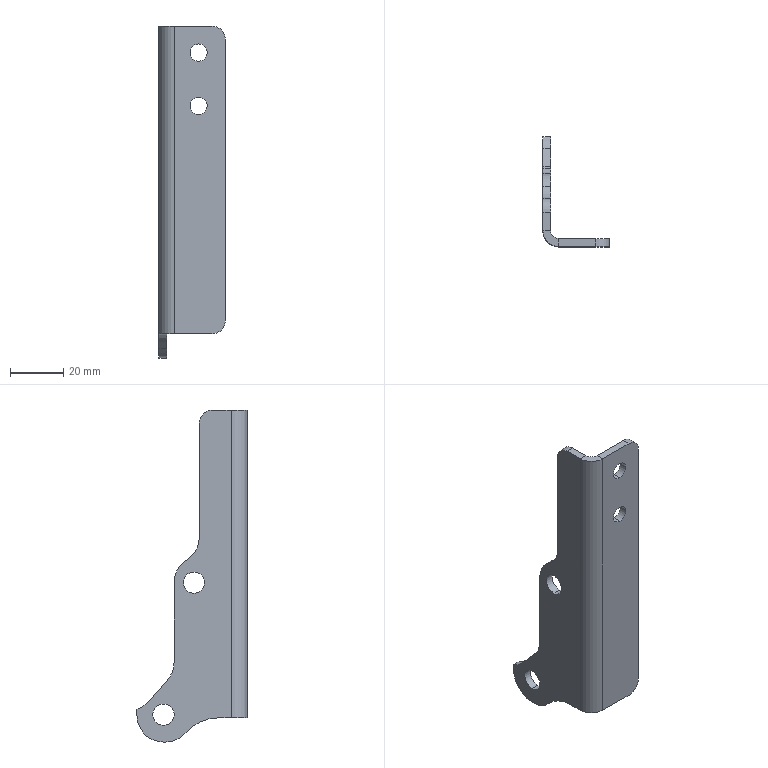Part | SolidWorks | features BaseBody 1 | 1 solid | 37 faces | box 25 x 41.473 x 125 mm | volume 15257 mm3 | cylinder 21 | plane 16 | commonest cylinder face diameters 20 x6 6.5 x4 8 x4 10 x3 6 x1 12 x1
STEP:
#1=CARTESIAN_POINT('',(0.,30.37,-102.09));
#2=VERTEX_POINT('',#1);
#3=CARTESIAN_POINT('',(3.,30.37,-102.09));
#4=VERTEX_POINT('',#3);
#5=CARTESIAN_POINT('',(3.,30.37,-102.09));
#6=DIRECTION('',(1.,0.,0.));
#7=VECTOR('',#6,1000.);
#8=LINE('',#5,#7);
#9=EDGE_CURVE('',#2,#4,#8,.T.);
#10=ORIENTED_EDGE('',*,*,#9,.T.);
#11=CARTESIAN_POINT('',(3.,37.101,-109.825));
#12=VERTEX_POINT('',#11);
#13=CARTESIAN_POINT('',(3.,28.627,-100.088));
#14=DIRECTION('',(0.,0.6565,-0.7544));
#15=VECTOR('',#14,1000.);
#16=LINE('',#13,#15);
#17=EDGE_CURVE('',#4,#12,#16,.T.);
#18=ORIENTED_EDGE('',*,*,#17,.T.);
#19=CARTESIAN_POINT('',(0.,37.101,-109.825));
#20=VERTEX_POINT('',#19);
#21=CARTESIAN_POINT('',(10.,37.101,-109.825));
#22=DIRECTION('',(-1.,0.,0.));
#23=VECTOR('',#22,1000.);
#24=LINE('',#21,#23);
#25=EDGE_CURVE('',#12,#20,#24,.T.);
#26=ORIENTED_EDGE('',*,*,#25,.T.);
#27=CARTESIAN_POINT('',(0.,29.519,-101.113));
#28=DIRECTION('',(0.,0.6565,-0.7544));
#29=VECTOR('',#28,1000.);
#30=LINE('',#27,#29);
#31=EDGE_CURVE('',#2,#20,#30,.T.);
#32=ORIENTED_EDGE('',*,*,#31,.F.);
#33=EDGE_LOOP('',(#10,#18,#26,#32));
#34=FACE_OUTER_BOUND('',#33,.T.);
#35=CARTESIAN_POINT('',(10.,29.519,-101.113));
#36=DIRECTION('',(0.,-0.7544,-0.6565));
#37=DIRECTION('',(0.,0.6565,-0.7544));
#38=AXIS2_PLACEMENT_3D('',#35,#36,#37);
#39=PLANE('',#38);
#40=ADVANCED_FACE('',(#34),#39,.F.);
#41=CARTESIAN_POINT('',(0.,18.,-5.));
#42=VERTEX_POINT('',#41);
#43=CARTESIAN_POINT('',(0.,13.,0.));
#44=VERTEX_POINT('',#43);
#45=CARTESIAN_POINT('',(0.,13.,-5.));
#46=DIRECTION('',(1.,0.,0.));
#47=DIRECTION('',(0.,0.,-1.));
#48=AXIS2_PLACEMENT_3D('',#45,#46,#47);
#49=CIRCLE('',#48,5.);
#50=EDGE_CURVE('',#42,#44,#49,.T.);
#51=ORIENTED_EDGE('',*,*,#50,.T.);
#52=CARTESIAN_POINT('',(3.,13.,0.));
#53=VERTEX_POINT('',#52);
#54=CARTESIAN_POINT('',(6.,13.,0.));
#55=DIRECTION('',(1.,0.,0.));
#56=VECTOR('',#55,1000.);
#57=LINE('',#54,#56);
#58=EDGE_CURVE('',#44,#53,#57,.T.);
#59=ORIENTED_EDGE('',*,*,#58,.T.);
#60=CARTESIAN_POINT('',(3.,18.,-5.));
#61=VERTEX_POINT('',#60);
#62=CARTESIAN_POINT('',(3.,13.,-5.));
#63=DIRECTION('',(-1.,0.,0.));
#64=DIRECTION('',(0.,0.,-1.));
#65=AXIS2_PLACEMENT_3D('',#62,#63,#64);
#66=CIRCLE('',#65,5.);
#67=EDGE_CURVE('',#53,#61,#66,.T.);
#68=ORIENTED_EDGE('',*,*,#67,.T.);
#69=CARTESIAN_POINT('',(-7.,18.,-5.));
#70=DIRECTION('',(-1.,0.,0.));
#71=VECTOR('',#70,1000.);
#72=LINE('',#69,#71);
#73=EDGE_CURVE('',#61,#42,#72,.T.);
#74=ORIENTED_EDGE('',*,*,#73,.T.);
#75=EDGE_LOOP('',(#51,#59,#68,#74));
#76=FACE_OUTER_BOUND('',#75,.T.);
#77=CARTESIAN_POINT('',(6.,13.,-5.));
#78=DIRECTION('',(1.,0.,0.));
#79=DIRECTION('',(0.,0.,1.));
#80=AXIS2_PLACEMENT_3D('',#77,#78,#79);
#81=CYLINDRICAL_SURFACE('',#80,5.);
#82=ADVANCED_FACE('',(#76),#81,.T.);
#83=CARTESIAN_POINT('',(25.,3.,-5.));
#84=VERTEX_POINT('',#83);
#85=CARTESIAN_POINT('',(20.,3.,0.));
#86=VERTEX_POINT('',#85);
#87=CARTESIAN_POINT('',(20.,3.,-5.));
#88=DIRECTION('',(0.,-1.,0.));
#89=DIRECTION('',(0.,0.,1.));
#90=AXIS2_PLACEMENT_3D('',#87,#88,#89);
#91=CIRCLE('',#90,5.);
#92=EDGE_CURVE('',#84,#86,#91,.T.);
#93=ORIENTED_EDGE('',*,*,#92,.T.);
#94=CARTESIAN_POINT('',(20.,0.,0.));
#95=VERTEX_POINT('',#94);
#96=CARTESIAN_POINT('',(20.,6.,0.));
#97=DIRECTION('',(0.,-1.,0.));
#98=VECTOR('',#97,1000.);
#99=LINE('',#96,#98);
#100=EDGE_CURVE('',#86,#95,#99,.T.);
#101=ORIENTED_EDGE('',*,*,#100,.T.);
#102=CARTESIAN_POINT('',(25.,0.,-5.));
#103=VERTEX_POINT('',#102);
#104=CARTESIAN_POINT('',(20.,0.,-5.));
#105=DIRECTION('',(0.,1.,0.));
#106=DIRECTION('',(0.,0.,1.));
#107=AXIS2_PLACEMENT_3D('',#104,#105,#106);
#108=CIRCLE('',#107,5.);
#109=EDGE_CURVE('',#95,#103,#108,.T.);
#110=ORIENTED_EDGE('',*,*,#109,.T.);
#111=CARTESIAN_POINT('',(25.,3.,-5.));
#112=DIRECTION('',(0.,1.,0.));
#113=VECTOR('',#112,1000.);
#114=LINE('',#111,#113);
#115=EDGE_CURVE('',#103,#84,#114,.T.);
#116=ORIENTED_EDGE('',*,*,#115,.T.);
#117=EDGE_LOOP('',(#93,#101,#110,#116));
#118=FACE_OUTER_BOUND('',#117,.T.);
#119=CARTESIAN_POINT('',(20.,6.,-5.));
#120=DIRECTION('',(0.,-1.,0.));
#121=DIRECTION('',(0.,0.,1.));
#122=AXIS2_PLACEMENT_3D('',#119,#120,#121);
#123=CYLINDRICAL_SURFACE('',#122,5.);
#124=ADVANCED_FACE('',(#118),#123,.T.);
#125=CARTESIAN_POINT('',(20.,3.,-115.955));
#126=VERTEX_POINT('',#125);
#127=CARTESIAN_POINT('',(25.,3.,-110.955));
#128=VERTEX_POINT('',#127);
#129=CARTESIAN_POINT('',(20.,3.,-110.955));
#130=DIRECTION('',(0.,-1.,0.));
#131=DIRECTION('',(0.,0.,1.));
#132=AXIS2_PLACEMENT_3D('',#129,#130,#131);
#133=CIRCLE('',#132,5.);
#134=EDGE_CURVE('',#126,#128,#133,.T.);
#135=ORIENTED_EDGE('',*,*,#134,.T.);
#136=CARTESIAN_POINT('',(25.,0.,-110.955));
#137=VERTEX_POINT('',#136);
#138=CARTESIAN_POINT('',(25.,3.,-110.955));
#139=DIRECTION('',(0.,-1.,0.));
#140=VECTOR('',#139,1000.);
#141=LINE('',#138,#140);
#142=EDGE_CURVE('',#128,#137,#141,.T.);
#143=ORIENTED_EDGE('',*,*,#142,.T.);
#144=CARTESIAN_POINT('',(20.,0.,-115.955));
#145=VERTEX_POINT('',#144);
#146=CARTESIAN_POINT('',(20.,0.,-110.955));
#147=DIRECTION('',(0.,1.,0.));
#148=DIRECTION('',(0.,0.,1.));
#149=AXIS2_PLACEMENT_3D('',#146,#147,#148);
#150=CIRCLE('',#149,5.);
#151=EDGE_CURVE('',#137,#145,#150,.T.);
#152=ORIENTED_EDGE('',*,*,#151,.T.);
#153=CARTESIAN_POINT('',(20.,3.,-115.955));
#154=DIRECTION('',(0.,1.,0.));
#155=VECTOR('',#154,1000.);
#156=LINE('',#153,#155);
#157=EDGE_CURVE('',#145,#126,#156,.T.);
#158=ORIENTED_EDGE('',*,*,#157,.T.);
#159=EDGE_LOOP('',(#135,#143,#152,#158));
#160=FACE_OUTER_BOUND('',#159,.T.);
#161=CARTESIAN_POINT('',(20.,3.,-110.955));
#162=DIRECTION('',(0.,1.,0.));
#163=DIRECTION('',(0.,0.,-1.));
#164=AXIS2_PLACEMENT_3D('',#161,#162,#163);
#165=CYLINDRICAL_SURFACE('',#164,5.);
#166=ADVANCED_FACE('',(#160),#165,.T.);
#167=CARTESIAN_POINT('',(0.,22.983,-121.487));
#168=VERTEX_POINT('',#167);
#169=CARTESIAN_POINT('',(0.,30.594,-125.));
#170=VERTEX_POINT('',#169);
#171=CARTESIAN_POINT('',(0.,30.594,-115.));
#172=DIRECTION('',(1.,0.,0.));
#173=DIRECTION('',(0.,0.,-1.));
#174=AXIS2_PLACEMENT_3D('',#171,#172,#173);
#175=CIRCLE('',#174,10.);
#176=EDGE_CURVE('',#168,#170,#175,.T.);
#177=ORIENTED_EDGE('',*,*,#176,.T.);
#178=CARTESIAN_POINT('',(3.,30.594,-125.));
#179=VERTEX_POINT('',#178);
#180=CARTESIAN_POINT('',(6.,30.594,-125.));
#181=DIRECTION('',(1.,0.,0.));
#182=VECTOR('',#181,1000.);
#183=LINE('',#180,#182);
#184=EDGE_CURVE('',#170,#179,#183,.T.);
#185=ORIENTED_EDGE('',*,*,#184,.T.);
#186=CARTESIAN_POINT('',(3.,22.983,-121.487));
#187=VERTEX_POINT('',#186);
#188=CARTESIAN_POINT('',(3.,30.594,-115.));
#189=DIRECTION('',(-1.,0.,0.));
#190=DIRECTION('',(0.,0.,-1.));
#191=AXIS2_PLACEMENT_3D('',#188,#189,#190);
#192=CIRCLE('',#191,10.);
#193=EDGE_CURVE('',#179,#187,#192,.T.);
#194=ORIENTED_EDGE('',*,*,#193,.T.);
#195=CARTESIAN_POINT('',(0.,22.983,-121.487));
#196=DIRECTION('',(-1.,0.,0.));
#197=VECTOR('',#196,1000.);
#198=LINE('',#195,#197);
#199=EDGE_CURVE('',#187,#168,#198,.T.);
#200=ORIENTED_EDGE('',*,*,#199,.T.);
#201=EDGE_LOOP('',(#177,#185,#194,#200));
#202=FACE_OUTER_BOUND('',#201,.T.);
#203=CARTESIAN_POINT('',(0.,30.594,-115.));
#204=DIRECTION('',(-1.,0.,0.));
#205=DIRECTION('',(0.,0.,-1.));
#206=AXIS2_PLACEMENT_3D('',#203,#204,#205);
#207=CYLINDRICAL_SURFACE('',#206,10.);
#208=ADVANCED_FACE('',(#202),#207,.T.);
#209=CARTESIAN_POINT('',(0.,31.473,-125.));
#210=VERTEX_POINT('',#209);
#211=CARTESIAN_POINT('',(0.,41.473,-115.));
#212=VERTEX_POINT('',#211);
#213=CARTESIAN_POINT('',(0.,31.473,-115.));
#214=DIRECTION('',(1.,0.,0.));
#215=DIRECTION('',(0.,0.,-1.));
#216=AXIS2_PLACEMENT_3D('',#213,#214,#215);
#217=CIRCLE('',#216,10.);
#218=EDGE_CURVE('',#210,#212,#217,.T.);
#219=ORIENTED_EDGE('',*,*,#218,.T.);
#220=CARTESIAN_POINT('',(3.,41.473,-115.));
#221=VERTEX_POINT('',#220);
#222=CARTESIAN_POINT('',(3.,41.473,-115.));
#223=DIRECTION('',(1.,0.,0.));
#224=VECTOR('',#223,1000.);
#225=LINE('',#222,#224);
#226=EDGE_CURVE('',#212,#221,#225,.T.);
#227=ORIENTED_EDGE('',*,*,#226,.T.);
#228=CARTESIAN_POINT('',(3.,31.473,-125.));
#229=VERTEX_POINT('',#228);
#230=CARTESIAN_POINT('',(3.,31.473,-115.));
#231=DIRECTION('',(-1.,0.,0.));
#232=DIRECTION('',(0.,0.,-1.));
#233=AXIS2_PLACEMENT_3D('',#230,#231,#232);
#234=CIRCLE('',#233,10.);
#235=EDGE_CURVE('',#221,#229,#234,.T.);
#236=ORIENTED_EDGE('',*,*,#235,.T.);
#237=CARTESIAN_POINT('',(0.,31.473,-125.));
#238=DIRECTION('',(-1.,0.,0.));
#239=VECTOR('',#238,1000.);
#240=LINE('',#237,#239);
#241=EDGE_CURVE('',#229,#210,#240,.T.);
#242=ORIENTED_EDGE('',*,*,#241,.T.);
#243=EDGE_LOOP('',(#219,#227,#236,#242));
#244=FACE_OUTER_BOUND('',#243,.T.);
#245=CARTESIAN_POINT('',(-7.,31.473,-115.));
#246=DIRECTION('',(-1.,0.,0.));
#247=DIRECTION('',(0.,0.,-1.));
#248=AXIS2_PLACEMENT_3D('',#245,#246,#247);
#249=CYLINDRICAL_SURFACE('',#248,10.);
#250=ADVANCED_FACE('',(#244),#249,.T.);
#251=CARTESIAN_POINT('',(0.,22.736,-56.484));
#252=VERTEX_POINT('',#251);
#253=CARTESIAN_POINT('',(0.,18.,-47.981));
#254=VERTEX_POINT('',#253);
#255=CARTESIAN_POINT('',(0.,28.,-47.981));
#256=DIRECTION('',(-1.,0.,0.));
#257=DIRECTION('',(0.,0.,-1.));
#258=AXIS2_PLACEMENT_3D('',#255,#256,#257);
#259=CIRCLE('',#258,10.);
#260=EDGE_CURVE('',#252,#254,#259,.T.);
#261=ORIENTED_EDGE('',*,*,#260,.T.);
#262=CARTESIAN_POINT('',(3.,18.,-47.981));
#263=VERTEX_POINT('',#262);
#264=CARTESIAN_POINT('',(-7.,18.,-47.981));
#265=DIRECTION('',(1.,0.,0.));
#266=VECTOR('',#265,1000.);
#267=LINE('',#264,#266);
#268=EDGE_CURVE('',#254,#263,#267,.T.);
#269=ORIENTED_EDGE('',*,*,#268,.T.);
#270=CARTESIAN_POINT('',(3.,22.736,-56.484));
#271=VERTEX_POINT('',#270);
#272=CARTESIAN_POINT('',(3.,28.,-47.981));
#273=DIRECTION('',(1.,0.,0.));
#274=DIRECTION('',(0.,0.,-1.));
#275=AXIS2_PLACEMENT_3D('',#272,#273,#274);
#276=CIRCLE('',#275,10.);
#277=EDGE_CURVE('',#263,#271,#276,.T.);
#278=ORIENTED_EDGE('',*,*,#277,.T.);
#279=CARTESIAN_POINT('',(-7.,22.736,-56.484));
#280=DIRECTION('',(-1.,0.,0.));
#281=VECTOR('',#280,1000.);
#282=LINE('',#279,#281);
#283=EDGE_CURVE('',#271,#252,#282,.T.);
#284=ORIENTED_EDGE('',*,*,#283,.T.);
#285=EDGE_LOOP('',(#261,#269,#278,#284));
#286=FACE_OUTER_BOUND('',#285,.T.);
#287=CARTESIAN_POINT('',(-7.,28.,-47.981));
#288=DIRECTION('',(1.,0.,0.));
#289=DIRECTION('',(0.,0.,1.));
#290=AXIS2_PLACEMENT_3D('',#287,#288,#289);
#291=CYLINDRICAL_SURFACE('',#290,10.);
#292=ADVANCED_FACE('',(#286),#291,.F.);
#293=CARTESIAN_POINT('',(3.,27.473,-64.986));
#294=VERTEX_POINT('',#293);
#295=CARTESIAN_POINT('',(3.,17.473,-64.986));
#296=DIRECTION('',(-1.,0.,0.));
#297=DIRECTION('',(0.,0.,-1.));
#298=AXIS2_PLACEMENT_3D('',#295,#296,#297);
#299=CIRCLE('',#298,10.);
#300=EDGE_CURVE('',#271,#294,#299,.T.);
#301=ORIENTED_EDGE('',*,*,#300,.T.);
#302=CARTESIAN_POINT('',(0.,27.473,-64.986));
#303=VERTEX_POINT('',#302);
#304=CARTESIAN_POINT('',(-7.,27.473,-64.986));
#305=DIRECTION('',(-1.,0.,0.));
#306=VECTOR('',#305,1000.);
#307=LINE('',#304,#306);
#308=EDGE_CURVE('',#294,#303,#307,.T.);
#309=ORIENTED_EDGE('',*,*,#308,.T.);
#310=CARTESIAN_POINT('',(0.,17.473,-64.986));
#311=DIRECTION('',(1.,0.,0.));
#312=DIRECTION('',(0.,0.,-1.));
#313=AXIS2_PLACEMENT_3D('',#310,#311,#312);
#314=CIRCLE('',#313,10.);
#315=EDGE_CURVE('',#303,#252,#314,.T.);
#316=ORIENTED_EDGE('',*,*,#315,.T.);
#317=ORIENTED_EDGE('',*,*,#283,.F.);
#318=EDGE_LOOP('',(#301,#309,#316,#317));
#319=FACE_OUTER_BOUND('',#318,.T.);
#320=CARTESIAN_POINT('',(-7.,17.473,-64.986));
#321=DIRECTION('',(1.,0.,0.));
#322=DIRECTION('',(0.,0.,1.));
#323=AXIS2_PLACEMENT_3D('',#320,#321,#322);
#324=CYLINDRICAL_SURFACE('',#323,10.);
#325=ADVANCED_FACE('',(#319),#324,.T.);
#326=CARTESIAN_POINT('',(0.,6.,-115.955));
#327=VERTEX_POINT('',#326);
#328=CARTESIAN_POINT('',(6.,0.,-115.955));
#329=VERTEX_POINT('',#328);
#330=CARTESIAN_POINT('',(6.,6.,-115.955));
#331=DIRECTION('',(0.,0.,1.));
#332=DIRECTION('',(-1.,0.,0.));
#333=AXIS2_PLACEMENT_3D('',#330,#331,#332);
#334=CIRCLE('',#333,6.);
#335=EDGE_CURVE('',#327,#329,#334,.T.);
#336=ORIENTED_EDGE('',*,*,#335,.F.);
#337=CARTESIAN_POINT('',(3.,6.,-115.955));
#338=VERTEX_POINT('',#337);
#339=CARTESIAN_POINT('',(0.,6.,-115.955));
#340=DIRECTION('',(1.,0.,0.));
#341=VECTOR('',#340,1000.);
#342=LINE('',#339,#341);
#343=EDGE_CURVE('',#327,#338,#342,.T.);
#344=ORIENTED_EDGE('',*,*,#343,.T.);
#345=CARTESIAN_POINT('',(6.,3.,-115.955));
#346=VERTEX_POINT('',#345);
#347=CARTESIAN_POINT('',(6.,6.,-115.955));
#348=DIRECTION('',(0.,0.,1.));
#349=DIRECTION('',(-1.,0.,0.));
#350=AXIS2_PLACEMENT_3D('',#347,#348,#349);
#351=CIRCLE('',#350,3.);
#352=EDGE_CURVE('',#338,#346,#351,.T.);
#353=ORIENTED_EDGE('',*,*,#352,.T.);
#354=CARTESIAN_POINT('',(6.,3.,-115.955));
#355=DIRECTION('',(0.,-1.,0.));
#356=VECTOR('',#355,1000.);
#357=LINE('',#354,#356);
#358=EDGE_CURVE('',#346,#329,#357,.T.);
#359=ORIENTED_EDGE('',*,*,#358,.T.);
#360=EDGE_LOOP('',(#336,#344,#353,#359));
#361=FACE_OUTER_BOUND('',#360,.T.);
#362=CARTESIAN_POINT('',(6.,6.,-115.955));
#363=DIRECTION('',(0.,0.,-1.));
#364=DIRECTION('',(0.,-1.,0.));
#365=AXIS2_PLACEMENT_3D('',#362,#363,#364);
#366=PLANE('',#365);
#367=ADVANCED_FACE('',(#361),#366,.T.);
#368=CARTESIAN_POINT('',(0.,0.,-115.955));
#369=DIRECTION('',(1.,0.,0.));
#370=VECTOR('',#369,1000.);
#371=LINE('',#368,#370);
#372=EDGE_CURVE('',#329,#145,#371,.T.);
#373=ORIENTED_EDGE('',*,*,#372,.F.);
#374=ORIENTED_EDGE('',*,*,#358,.F.);
#375=CARTESIAN_POINT('',(0.,3.,-115.955));
#376=DIRECTION('',(1.,0.,0.));
#377=VECTOR('',#376,1000.);
#378=LINE('',#375,#377);
#379=EDGE_CURVE('',#346,#126,#378,.T.);
#380=ORIENTED_EDGE('',*,*,#379,.T.);
#381=ORIENTED_EDGE('',*,*,#157,.F.);
#382=EDGE_LOOP('',(#373,#374,#380,#381));
#383=FACE_OUTER_BOUND('',#382,.T.);
#384=CARTESIAN_POINT('',(0.,3.,-115.955));
#385=DIRECTION('',(0.,0.,1.));
#386=DIRECTION('',(1.,0.,0.));
#387=AXIS2_PLACEMENT_3D('',#384,#385,#386);
#388=PLANE('',#387);
#389=ADVANCED_FACE('',(#383),#388,.F.);
#390=CARTESIAN_POINT('',(0.,11.,-115.955));
#391=VERTEX_POINT('',#390);
#392=CARTESIAN_POINT('',(0.,11.,-115.955));
#393=DIRECTION('',(0.,-1.,0.));
#394=VECTOR('',#393,1000.);
#395=LINE('',#392,#394);
#396=EDGE_CURVE('',#391,#327,#395,.T.);
#397=ORIENTED_EDGE('',*,*,#396,.F.);
#398=CARTESIAN_POINT('',(3.,11.,-115.955));
#399=VERTEX_POINT('',#398);
#400=CARTESIAN_POINT('',(0.,11.,-115.955));
#401=DIRECTION('',(1.,0.,0.));
#402=VECTOR('',#401,1000.);
#403=LINE('',#400,#402);
#404=EDGE_CURVE('',#391,#399,#403,.T.);
#405=ORIENTED_EDGE('',*,*,#404,.T.);
#406=CARTESIAN_POINT('',(3.,0.,-115.955));
#407=DIRECTION('',(0.,-1.,0.));
#408=VECTOR('',#407,1000.);
#409=LINE('',#406,#408);
#410=EDGE_CURVE('',#399,#338,#409,.T.);
#411=ORIENTED_EDGE('',*,*,#410,.T.);
#412=ORIENTED_EDGE('',*,*,#343,.F.);
#413=EDGE_LOOP('',(#397,#405,#411,#412));
#414=FACE_OUTER_BOUND('',#413,.T.);
#415=CARTESIAN_POINT('',(0.,11.,-115.955));
#416=DIRECTION('',(0.,0.,1.));
#417=DIRECTION('',(1.,0.,0.));
#418=AXIS2_PLACEMENT_3D('',#415,#416,#417);
#419=PLANE('',#418);
#420=ADVANCED_FACE('',(#414),#419,.F.);
#421=CARTESIAN_POINT('',(3.,18.,-55.));
#422=DIRECTION('',(0.,0.,1.));
#423=VECTOR('',#422,1000.);
#424=LINE('',#421,#423);
#425=EDGE_CURVE('',#263,#61,#424,.T.);
#426=ORIENTED_EDGE('',*,*,#425,.F.);
#427=ORIENTED_EDGE('',*,*,#268,.F.);
#428=CARTESIAN_POINT('',(0.,18.,-125.));
#429=DIRECTION('',(0.,0.,-1.));
#430=VECTOR('',#429,1000.);
#431=LINE('',#428,#430);
#432=EDGE_CURVE('',#42,#254,#431,.T.);
#433=ORIENTED_EDGE('',*,*,#432,.F.);
#434=ORIENTED_EDGE('',*,*,#73,.F.);
#435=EDGE_LOOP('',(#426,#427,#433,#434));
#436=FACE_OUTER_BOUND('',#435,.T.);
#437=CARTESIAN_POINT('',(-7.,18.,-55.));
#438=DIRECTION('',(0.,-1.,0.));
#439=DIRECTION('',(0.,0.,-1.));
#440=AXIS2_PLACEMENT_3D('',#437,#438,#439);
#441=PLANE('',#440);
#442=ADVANCED_FACE('',(#436),#441,.F.);
#443=CARTESIAN_POINT('',(15.,3.,-13.25));
#444=VERTEX_POINT('',#443);
#445=CARTESIAN_POINT('',(15.,0.,-13.25));
#446=VERTEX_POINT('',#445);
#447=CARTESIAN_POINT('',(15.,10.,-13.25));
#448=DIRECTION('',(0.,-1.,0.));
#449=VECTOR('',#448,1000.);
#450=LINE('',#447,#449);
#451=EDGE_CURVE('',#444,#446,#450,.T.);
#452=ORIENTED_EDGE('',*,*,#451,.F.);
#453=CARTESIAN_POINT('',(15.,3.,-6.75));
#454=VERTEX_POINT('',#453);
#455=CARTESIAN_POINT('',(15.,3.,-10.));
#456=DIRECTION('',(0.,1.,0.));
#457=DIRECTION('',(0.,0.,1.));
#458=AXIS2_PLACEMENT_3D('',#455,#456,#457);
#459=CIRCLE('',#458,3.25);
#460=EDGE_CURVE('',#444,#454,#459,.T.);
#461=ORIENTED_EDGE('',*,*,#460,.T.);
#462=CARTESIAN_POINT('',(15.,0.,-6.75));
#463=VERTEX_POINT('',#462);
#464=CARTESIAN_POINT('',(15.,10.,-6.75));
#465=DIRECTION('',(0.,-1.,0.));
#466=VECTOR('',#465,1000.);
#467=LINE('',#464,#466);
#468=EDGE_CURVE('',#454,#463,#467,.T.);
#469=ORIENTED_EDGE('',*,*,#468,.T.);
#470=CARTESIAN_POINT('',(15.,0.,-10.));
#471=DIRECTION('',(0.,1.,0.));
#472=DIRECTION('',(0.,0.,1.));
#473=AXIS2_PLACEMENT_3D('',#470,#471,#472);
#474=CIRCLE('',#473,3.25);
#475=EDGE_CURVE('',#446,#463,#474,.T.);
#476=ORIENTED_EDGE('',*,*,#475,.F.);
#477=EDGE_LOOP('',(#452,#461,#469,#476));
#478=FACE_OUTER_BOUND('',#477,.T.);
#479=CARTESIAN_POINT('',(15.,10.,-10.));
#480=DIRECTION('',(0.,-1.,0.));
#481=DIRECTION('',(0.,0.,1.));
#482=AXIS2_PLACEMENT_3D('',#479,#480,#481);
#483=CYLINDRICAL_SURFACE('',#482,3.25);
#484=ADVANCED_FACE('',(#478),#483,.F.);
#485=CARTESIAN_POINT('',(15.,3.,-33.25));
#486=VERTEX_POINT('',#485);
#487=CARTESIAN_POINT('',(15.,0.,-33.25));
#488=VERTEX_POINT('',#487);
#489=CARTESIAN_POINT('',(15.,10.,-33.25));
#490=DIRECTION('',(0.,-1.,0.));
#491=VECTOR('',#490,1000.);
#492=LINE('',#489,#491);
#493=EDGE_CURVE('',#486,#488,#492,.T.);
#494=ORIENTED_EDGE('',*,*,#493,.F.);
#495=CARTESIAN_POINT('',(15.,3.,-26.75));
#496=VERTEX_POINT('',#495);
#497=CARTESIAN_POINT('',(15.,3.,-30.));
#498=DIRECTION('',(0.,1.,0.));
#499=DIRECTION('',(0.,0.,1.));
#500=AXIS2_PLACEMENT_3D('',#497,#498,#499);
#501=CIRCLE('',#500,3.25);
#502=EDGE_CURVE('',#486,#496,#501,.T.);
#503=ORIENTED_EDGE('',*,*,#502,.T.);
#504=CARTESIAN_POINT('',(15.,0.,-26.75));
#505=VERTEX_POINT('',#504);
#506=CARTESIAN_POINT('',(15.,10.,-26.75));
#507=DIRECTION('',(0.,-1.,0.));
#508=VECTOR('',#507,1000.);
#509=LINE('',#506,#508);
#510=EDGE_CURVE('',#496,#505,#509,.T.);
#511=ORIENTED_EDGE('',*,*,#510,.T.);
#512=CARTESIAN_POINT('',(15.,0.,-30.));
#513=DIRECTION('',(0.,1.,0.));
#514=DIRECTION('',(0.,0.,1.));
#515=AXIS2_PLACEMENT_3D('',#512,#513,#514);
#516=CIRCLE('',#515,3.25);
#517=EDGE_CURVE('',#488,#505,#516,.T.);
#518=ORIENTED_EDGE('',*,*,#517,.F.);
#519=EDGE_LOOP('',(#494,#503,#511,#518));
#520=FACE_OUTER_BOUND('',#519,.T.);
#521=CARTESIAN_POINT('',(15.,10.,-30.));
#522=DIRECTION('',(0.,-1.,0.));
#523=DIRECTION('',(0.,0.,1.));
#524=AXIS2_PLACEMENT_3D('',#521,#522,#523);
#525=CYLINDRICAL_SURFACE('',#524,3.25);
#526=ADVANCED_FACE('',(#520),#525,.F.);
#527=CARTESIAN_POINT('',(0.,29.519,-101.113));
#528=VERTEX_POINT('',#527);
#529=CARTESIAN_POINT('',(0.,37.473,-95.051));
#530=DIRECTION('',(-1.,0.,0.));
#531=DIRECTION('',(0.,0.,-1.));
#532=AXIS2_PLACEMENT_3D('',#529,#530,#531);
#533=CIRCLE('',#532,10.);
#534=EDGE_CURVE('',#2,#528,#533,.T.);
#535=ORIENTED_EDGE('',*,*,#534,.T.);
#536=CARTESIAN_POINT('',(3.,29.519,-101.113));
#537=VERTEX_POINT('',#536);
#538=CARTESIAN_POINT('',(3.,29.519,-101.113));
#539=DIRECTION('',(-1.,0.,0.));
#540=VECTOR('',#539,1000.);
#541=LINE('',#538,#540);
#542=EDGE_CURVE('',#537,#528,#541,.T.);
#543=ORIENTED_EDGE('',*,*,#542,.F.);
#544=CARTESIAN_POINT('',(3.,37.473,-95.051));
#545=DIRECTION('',(1.,0.,0.));
#546=DIRECTION('',(0.,0.,-1.));
#547=AXIS2_PLACEMENT_3D('',#544,#545,#546);
#548=CIRCLE('',#547,10.);
#549=EDGE_CURVE('',#537,#4,#548,.T.);
#550=ORIENTED_EDGE('',*,*,#549,.T.);
#551=ORIENTED_EDGE('',*,*,#9,.F.);
#552=EDGE_LOOP('',(#535,#543,#550,#551));
#553=FACE_OUTER_BOUND('',#552,.T.);
#554=CARTESIAN_POINT('',(3.,37.473,-95.051));
#555=DIRECTION('',(-1.,0.,0.));
#556=DIRECTION('',(0.,0.,-1.));
#557=AXIS2_PLACEMENT_3D('',#554,#555,#556);
#558=CYLINDRICAL_SURFACE('',#557,10.);
#559=ADVANCED_FACE('',(#553),#558,.F.);
#560=CARTESIAN_POINT('',(3.,31.473,-110.693));
#561=VERTEX_POINT('',#560);
#562=CARTESIAN_POINT('',(0.,31.473,-110.693));
#563=VERTEX_POINT('',#562);
#564=CARTESIAN_POINT('',(10.,31.473,-110.693));
#565=DIRECTION('',(-1.,0.,0.));
#566=VECTOR('',#565,1000.);
#567=LINE('',#564,#566);
#568=EDGE_CURVE('',#561,#563,#567,.T.);
#569=ORIENTED_EDGE('',*,*,#568,.F.);
#570=CARTESIAN_POINT('',(3.,31.473,-118.693));
#571=VERTEX_POINT('',#570);
#572=CARTESIAN_POINT('',(3.,31.473,-114.693));
#573=DIRECTION('',(1.,0.,0.));
#574=DIRECTION('',(0.,0.,-1.));
#575=AXIS2_PLACEMENT_3D('',#572,#573,#574);
#576=CIRCLE('',#575,4.);
#577=EDGE_CURVE('',#561,#571,#576,.T.);
#578=ORIENTED_EDGE('',*,*,#577,.T.);
#579=CARTESIAN_POINT('',(0.,31.473,-118.693));
#580=VERTEX_POINT('',#579);
#581=CARTESIAN_POINT('',(10.,31.473,-118.693));
#582=DIRECTION('',(-1.,0.,0.));
#583=VECTOR('',#582,1000.);
#584=LINE('',#581,#583);
#585=EDGE_CURVE('',#571,#580,#584,.T.);
#586=ORIENTED_EDGE('',*,*,#585,.T.);
#587=CARTESIAN_POINT('',(0.,31.473,-114.693));
#588=DIRECTION('',(1.,0.,0.));
#589=DIRECTION('',(0.,0.,-1.));
#590=AXIS2_PLACEMENT_3D('',#587,#588,#589);
#591=CIRCLE('',#590,4.);
#592=EDGE_CURVE('',#563,#580,#591,.T.);
#593=ORIENTED_EDGE('',*,*,#592,.F.);
#594=EDGE_LOOP('',(#569,#578,#586,#593));
#595=FACE_OUTER_BOUND('',#594,.T.);
#596=CARTESIAN_POINT('',(10.,31.473,-114.693));
#597=DIRECTION('',(-1.,0.,0.));
#598=DIRECTION('',(0.,0.,-1.));
#599=AXIS2_PLACEMENT_3D('',#596,#597,#598);
#600=CYLINDRICAL_SURFACE('',#599,4.);
#601=ADVANCED_FACE('',(#595),#600,.F.);
#602=CARTESIAN_POINT('',(3.,20.,-61.));
#603=VERTEX_POINT('',#602);
#604=CARTESIAN_POINT('',(0.,20.,-61.));
#605=VERTEX_POINT('',#604);
#606=CARTESIAN_POINT('',(10.,20.,-61.));
#607=DIRECTION('',(-1.,0.,0.));
#608=VECTOR('',#607,1000.);
#609=LINE('',#606,#608);
#610=EDGE_CURVE('',#603,#605,#609,.T.);
#611=ORIENTED_EDGE('',*,*,#610,.F.);
#612=CARTESIAN_POINT('',(3.,20.,-69.));
#613=VERTEX_POINT('',#612);
#614=CARTESIAN_POINT('',(3.,20.,-65.));
#615=DIRECTION('',(1.,0.,0.));
#616=DIRECTION('',(0.,0.,-1.));
#617=AXIS2_PLACEMENT_3D('',#614,#615,#616);
#618=CIRCLE('',#617,4.);
#619=EDGE_CURVE('',#603,#613,#618,.T.);
#620=ORIENTED_EDGE('',*,*,#619,.T.);
#621=CARTESIAN_POINT('',(0.,20.,-69.));
#622=VERTEX_POINT('',#621);
#623=CARTESIAN_POINT('',(10.,20.,-69.));
#624=DIRECTION('',(-1.,0.,0.));
#625=VECTOR('',#624,1000.);
#626=LINE('',#623,#625);
#627=EDGE_CURVE('',#613,#622,#626,.T.);
#628=ORIENTED_EDGE('',*,*,#627,.T.);
#629=CARTESIAN_POINT('',(0.,20.,-65.));
#630=DIRECTION('',(1.,0.,0.));
#631=DIRECTION('',(0.,0.,-1.));
#632=AXIS2_PLACEMENT_3D('',#629,#630,#631);
#633=CIRCLE('',#632,4.);
#634=EDGE_CURVE('',#605,#622,#633,.T.);
#635=ORIENTED_EDGE('',*,*,#634,.F.);
#636=EDGE_LOOP('',(#611,#620,#628,#635));
#637=FACE_OUTER_BOUND('',#636,.T.);
#638=CARTESIAN_POINT('',(10.,20.,-65.));
#639=DIRECTION('',(-1.,0.,0.));
#640=DIRECTION('',(0.,0.,-1.));
#641=AXIS2_PLACEMENT_3D('',#638,#639,#640);
#642=CYLINDRICAL_SURFACE('',#641,4.);
#643=ADVANCED_FACE('',(#637),#642,.F.);
#644=CARTESIAN_POINT('',(0.,6.,0.));
#645=VERTEX_POINT('',#644);
#646=CARTESIAN_POINT('',(0.,0.,0.));
#647=DIRECTION('',(0.,1.,0.));
#648=VECTOR('',#647,1000.);
#649=LINE('',#646,#648);
#650=EDGE_CURVE('',#645,#44,#649,.T.);
#651=ORIENTED_EDGE('',*,*,#650,.F.);
#652=CARTESIAN_POINT('',(3.,6.,0.));
#653=VERTEX_POINT('',#652);
#654=CARTESIAN_POINT('',(3.,6.,0.));
#655=DIRECTION('',(-1.,0.,0.));
#656=VECTOR('',#655,1000.);
#657=LINE('',#654,#656);
#658=EDGE_CURVE('',#653,#645,#657,.T.);
#659=ORIENTED_EDGE('',*,*,#658,.F.);
#660=CARTESIAN_POINT('',(3.,0.,0.));
#661=DIRECTION('',(0.,1.,0.));
#662=VECTOR('',#661,1000.);
#663=LINE('',#660,#662);
#664=EDGE_CURVE('',#653,#53,#663,.T.);
#665=ORIENTED_EDGE('',*,*,#664,.T.);
#666=ORIENTED_EDGE('',*,*,#58,.F.);
#667=EDGE_LOOP('',(#651,#659,#665,#666));
#668=FACE_OUTER_BOUND('',#667,.T.);
#669=CARTESIAN_POINT('',(6.,6.,0.));
#670=DIRECTION('',(0.,0.,-1.));
#671=DIRECTION('',(0.,-1.,0.));
#672=AXIS2_PLACEMENT_3D('',#669,#670,#671);
#673=PLANE('',#672);
#674=ADVANCED_FACE('',(#668),#673,.F.);
#675=CARTESIAN_POINT('',(6.,3.,0.));
#676=VERTEX_POINT('',#675);
#677=CARTESIAN_POINT('',(0.,3.,0.));
#678=DIRECTION('',(-1.,0.,0.));
#679=VECTOR('',#678,1000.);
#680=LINE('',#677,#679);
#681=EDGE_CURVE('',#86,#676,#680,.T.);
#682=ORIENTED_EDGE('',*,*,#681,.T.);
#683=CARTESIAN_POINT('',(6.,0.,0.));
#684=VERTEX_POINT('',#683);
#685=CARTESIAN_POINT('',(6.,0.,0.));
#686=DIRECTION('',(0.,1.,0.));
#687=VECTOR('',#686,1000.);
#688=LINE('',#685,#687);
#689=EDGE_CURVE('',#684,#676,#688,.T.);
#690=ORIENTED_EDGE('',*,*,#689,.F.);
#691=CARTESIAN_POINT('',(0.,0.,0.));
#692=DIRECTION('',(-1.,0.,0.));
#693=VECTOR('',#692,1000.);
#694=LINE('',#691,#693);
#695=EDGE_CURVE('',#95,#684,#694,.T.);
#696=ORIENTED_EDGE('',*,*,#695,.F.);
#697=ORIENTED_EDGE('',*,*,#100,.F.);
#698=EDGE_LOOP('',(#682,#690,#696,#697));
#699=FACE_OUTER_BOUND('',#698,.T.);
#700=CARTESIAN_POINT('',(3.,6.,0.));
#701=DIRECTION('',(0.,0.,1.));
#702=DIRECTION('',(1.,0.,0.));
#703=AXIS2_PLACEMENT_3D('',#700,#701,#702);
#704=PLANE('',#703);
#705=ADVANCED_FACE('',(#699),#704,.T.);
#706=ORIENTED_EDGE('',*,*,#689,.T.);
#707=CARTESIAN_POINT('',(6.,6.,0.));
#708=DIRECTION('',(0.,0.,-1.));
#709=DIRECTION('',(1.,0.,0.));
#710=AXIS2_PLACEMENT_3D('',#707,#708,#709);
#711=CIRCLE('',#710,3.);
#712=EDGE_CURVE('',#676,#653,#711,.T.);
#713=ORIENTED_EDGE('',*,*,#712,.T.);
#714=ORIENTED_EDGE('',*,*,#658,.T.);
#715=CARTESIAN_POINT('',(6.,6.,0.));
#716=DIRECTION('',(0.,0.,-1.));
#717=DIRECTION('',(1.,0.,0.));
#718=AXIS2_PLACEMENT_3D('',#715,#716,#717);
#719=CIRCLE('',#718,6.);
#720=EDGE_CURVE('',#684,#645,#719,.T.);
#721=ORIENTED_EDGE('',*,*,#720,.F.);
#722=EDGE_LOOP('',(#706,#713,#714,#721));
#723=FACE_OUTER_BOUND('',#722,.T.);
#724=CARTESIAN_POINT('',(6.,0.,0.));
#725=DIRECTION('',(0.,0.,1.));
#726=DIRECTION('',(1.,0.,0.));
#727=AXIS2_PLACEMENT_3D('',#724,#725,#726);
#728=PLANE('',#727);
#729=ADVANCED_FACE('',(#723),#728,.T.);
#730=CARTESIAN_POINT('',(3.,27.473,-95.051));
#731=VERTEX_POINT('',#730);
#732=CARTESIAN_POINT('',(3.,27.473,-104.693));
#733=DIRECTION('',(0.,0.,1.));
#734=VECTOR('',#733,1000.);
#735=LINE('',#732,#734);
#736=EDGE_CURVE('',#731,#294,#735,.T.);
#737=ORIENTED_EDGE('',*,*,#736,.F.);
#738=CARTESIAN_POINT('',(0.,27.473,-95.051));
#739=VERTEX_POINT('',#738);
#740=CARTESIAN_POINT('',(-7.,27.473,-95.051));
#741=DIRECTION('',(1.,0.,0.));
#742=VECTOR('',#741,1000.);
#743=LINE('',#740,#742);
#744=EDGE_CURVE('',#739,#731,#743,.T.);
#745=ORIENTED_EDGE('',*,*,#744,.F.);
#746=CARTESIAN_POINT('',(0.,27.473,-125.));
#747=DIRECTION('',(0.,0.,-1.));
#748=VECTOR('',#747,1000.);
#749=LINE('',#746,#748);
#750=EDGE_CURVE('',#303,#739,#749,.T.);
#751=ORIENTED_EDGE('',*,*,#750,.F.);
#752=ORIENTED_EDGE('',*,*,#308,.F.);
#753=EDGE_LOOP('',(#737,#745,#751,#752));
#754=FACE_OUTER_BOUND('',#753,.T.);
#755=CARTESIAN_POINT('',(-7.,27.473,-104.693));
#756=DIRECTION('',(0.,-1.,0.));
#757=DIRECTION('',(0.,0.,-1.));
#758=AXIS2_PLACEMENT_3D('',#755,#756,#757);
#759=PLANE('',#758);
#760=ADVANCED_FACE('',(#754),#759,.F.);
#761=CARTESIAN_POINT('',(0.,41.473,-112.677));
#762=VERTEX_POINT('',#761);
#763=CARTESIAN_POINT('',(0.,41.473,-125.));
#764=DIRECTION('',(0.,0.,-1.));
#765=VECTOR('',#764,1000.);
#766=LINE('',#763,#765);
#767=EDGE_CURVE('',#762,#212,#766,.T.);
#768=ORIENTED_EDGE('',*,*,#767,.F.);
#769=CARTESIAN_POINT('',(3.,41.473,-112.677));
#770=VERTEX_POINT('',#769);
#771=CARTESIAN_POINT('',(3.,41.473,-112.677));
#772=DIRECTION('',(-1.,0.,0.));
#773=VECTOR('',#772,1000.);
#774=LINE('',#771,#773);
#775=EDGE_CURVE('',#770,#762,#774,.T.);
#776=ORIENTED_EDGE('',*,*,#775,.F.);
#777=CARTESIAN_POINT('',(3.,41.473,0.));
#778=DIRECTION('',(0.,0.,1.));
#779=VECTOR('',#778,1000.);
#780=LINE('',#777,#779);
#781=EDGE_CURVE('',#221,#770,#780,.T.);
#782=ORIENTED_EDGE('',*,*,#781,.F.);
#783=ORIENTED_EDGE('',*,*,#226,.F.);
#784=EDGE_LOOP('',(#768,#776,#782,#783));
#785=FACE_OUTER_BOUND('',#784,.T.);
#786=CARTESIAN_POINT('',(-7.,41.473,0.));
#787=DIRECTION('',(0.,-1.,0.));
#788=DIRECTION('',(-1.,0.,0.));
#789=AXIS2_PLACEMENT_3D('',#786,#787,#788);
#790=PLANE('',#789);
#791=ADVANCED_FACE('',(#785),#790,.F.);
#792=CARTESIAN_POINT('',(3.,0.,-125.));
#793=DIRECTION('',(0.,1.,0.));
#794=VECTOR('',#793,1000.);
#795=LINE('',#792,#794);
#796=EDGE_CURVE('',#179,#229,#795,.T.);
#797=ORIENTED_EDGE('',*,*,#796,.F.);
#798=ORIENTED_EDGE('',*,*,#184,.F.);
#799=CARTESIAN_POINT('',(0.,0.,-125.));
#800=DIRECTION('',(0.,1.,0.));
#801=VECTOR('',#800,1000.);
#802=LINE('',#799,#801);
#803=EDGE_CURVE('',#170,#210,#802,.T.);
#804=ORIENTED_EDGE('',*,*,#803,.T.);
#805=ORIENTED_EDGE('',*,*,#241,.F.);
#806=EDGE_LOOP('',(#797,#798,#804,#805));
#807=FACE_OUTER_BOUND('',#806,.T.);
#808=CARTESIAN_POINT('',(6.,3.,-125.));
#809=DIRECTION('',(0.,0.,-1.));
#810=DIRECTION('',(0.,-1.,0.));
#811=AXIS2_PLACEMENT_3D('',#808,#809,#810);
#812=PLANE('',#811);
#813=ADVANCED_FACE('',(#807),#812,.T.);
#814=CARTESIAN_POINT('',(3.,11.,-131.7));
#815=DIRECTION('',(-1.,0.,0.));
#816=DIRECTION('',(0.,0.,1.));
#817=AXIS2_PLACEMENT_3D('',#814,#815,#816);
#818=CIRCLE('',#817,15.745);
#819=EDGE_CURVE('',#399,#187,#818,.T.);
#820=ORIENTED_EDGE('',*,*,#819,.F.);
#821=ORIENTED_EDGE('',*,*,#404,.F.);
#822=CARTESIAN_POINT('',(0.,11.,-131.7));
#823=DIRECTION('',(-1.,0.,0.));
#824=DIRECTION('',(0.,0.,1.));
#825=AXIS2_PLACEMENT_3D('',#822,#823,#824);
#826=CIRCLE('',#825,15.745);
#827=EDGE_CURVE('',#391,#168,#826,.T.);
#828=ORIENTED_EDGE('',*,*,#827,.T.);
#829=ORIENTED_EDGE('',*,*,#199,.F.);
#830=EDGE_LOOP('',(#820,#821,#828,#829));
#831=FACE_OUTER_BOUND('',#830,.T.);
#832=CARTESIAN_POINT('',(0.,11.,-131.7));
#833=DIRECTION('',(-1.,0.,0.));
#834=DIRECTION('',(0.,0.,-1.));
#835=AXIS2_PLACEMENT_3D('',#832,#833,#834);
#836=CYLINDRICAL_SURFACE('',#835,15.745);
#837=ADVANCED_FACE('',(#831),#836,.F.);
#838=ORIENTED_EDGE('',*,*,#352,.F.);
#839=CARTESIAN_POINT('',(3.,6.,-125.));
#840=DIRECTION('',(0.,0.,1.));
#841=VECTOR('',#840,1000.);
#842=LINE('',#839,#841);
#843=EDGE_CURVE('',#338,#653,#842,.T.);
#844=ORIENTED_EDGE('',*,*,#843,.T.);
#845=ORIENTED_EDGE('',*,*,#712,.F.);
#846=CARTESIAN_POINT('',(6.,3.,-125.));
#847=DIRECTION('',(0.,0.,1.));
#848=VECTOR('',#847,1000.);
#849=LINE('',#846,#848);
#850=EDGE_CURVE('',#346,#676,#849,.T.);
#851=ORIENTED_EDGE('',*,*,#850,.F.);
#852=EDGE_LOOP('',(#838,#844,#845,#851));
#853=FACE_OUTER_BOUND('',#852,.T.);
#854=CARTESIAN_POINT('',(6.,6.,-125.));
#855=DIRECTION('',(0.,0.,1.));
#856=DIRECTION('',(-1.,0.,0.));
#857=AXIS2_PLACEMENT_3D('',#854,#855,#856);
#858=CYLINDRICAL_SURFACE('',#857,3.);
#859=ADVANCED_FACE('',(#853),#858,.F.);
#860=CARTESIAN_POINT('',(15.,3.,-10.));
#861=DIRECTION('',(0.,1.,0.));
#862=DIRECTION('',(0.,0.,1.));
#863=AXIS2_PLACEMENT_3D('',#860,#861,#862);
#864=CIRCLE('',#863,3.25);
#865=EDGE_CURVE('',#454,#444,#864,.T.);
#866=ORIENTED_EDGE('',*,*,#865,.F.);
#867=ORIENTED_EDGE('',*,*,#460,.F.);
#868=EDGE_LOOP('',(#866,#867));
#869=FACE_BOUND('',#868,.T.);
#870=CARTESIAN_POINT('',(15.,3.,-30.));
#871=DIRECTION('',(0.,1.,0.));
#872=DIRECTION('',(0.,0.,1.));
#873=AXIS2_PLACEMENT_3D('',#870,#871,#872);
#874=CIRCLE('',#873,3.25);
#875=EDGE_CURVE('',#496,#486,#874,.T.);
#876=ORIENTED_EDGE('',*,*,#875,.F.);
#877=ORIENTED_EDGE('',*,*,#502,.F.);
#878=EDGE_LOOP('',(#876,#877));
#879=FACE_BOUND('',#878,.T.);
#880=ORIENTED_EDGE('',*,*,#379,.F.);
#881=ORIENTED_EDGE('',*,*,#850,.T.);
#882=ORIENTED_EDGE('',*,*,#681,.F.);
#883=ORIENTED_EDGE('',*,*,#92,.F.);
#884=CARTESIAN_POINT('',(25.,3.,-125.));
#885=DIRECTION('',(0.,0.,1.));
#886=VECTOR('',#885,1000.);
#887=LINE('',#884,#886);
#888=EDGE_CURVE('',#128,#84,#887,.T.);
#889=ORIENTED_EDGE('',*,*,#888,.F.);
#890=ORIENTED_EDGE('',*,*,#134,.F.);
#891=EDGE_LOOP('',(#880,#881,#882,#883,#889,#890));
#892=FACE_OUTER_BOUND('',#891,.T.);
#893=CARTESIAN_POINT('',(0.,3.,-125.));
#894=DIRECTION('',(0.,-1.,0.));
#895=DIRECTION('',(0.,0.,-1.));
#896=AXIS2_PLACEMENT_3D('',#893,#894,#895);
#897=PLANE('',#896);
#898=ADVANCED_FACE('',(#869,#879,#892),#897,.F.);
#899=ORIENTED_EDGE('',*,*,#888,.T.);
#900=ORIENTED_EDGE('',*,*,#115,.F.);
#901=CARTESIAN_POINT('',(25.,0.,-125.));
#902=DIRECTION('',(0.,0.,1.));
#903=VECTOR('',#902,1000.);
#904=LINE('',#901,#903);
#905=EDGE_CURVE('',#137,#103,#904,.T.);
#906=ORIENTED_EDGE('',*,*,#905,.F.);
#907=ORIENTED_EDGE('',*,*,#142,.F.);
#908=EDGE_LOOP('',(#899,#900,#906,#907));
#909=FACE_OUTER_BOUND('',#908,.T.);
#910=CARTESIAN_POINT('',(25.,3.,-125.));
#911=DIRECTION('',(1.,0.,0.));
#912=DIRECTION('',(0.,1.,0.));
#913=AXIS2_PLACEMENT_3D('',#910,#911,#912);
#914=PLANE('',#913);
#915=ADVANCED_FACE('',(#909),#914,.T.);
#916=CARTESIAN_POINT('',(15.,0.,-30.));
#917=DIRECTION('',(0.,1.,0.));
#918=DIRECTION('',(0.,0.,1.));
#919=AXIS2_PLACEMENT_3D('',#916,#917,#918);
#920=CIRCLE('',#919,3.25);
#921=EDGE_CURVE('',#505,#488,#920,.T.);
#922=ORIENTED_EDGE('',*,*,#921,.T.);
#923=ORIENTED_EDGE('',*,*,#517,.T.);
#924=EDGE_LOOP('',(#922,#923));
#925=FACE_BOUND('',#924,.T.);
#926=CARTESIAN_POINT('',(15.,0.,-10.));
#927=DIRECTION('',(0.,1.,0.));
#928=DIRECTION('',(0.,0.,1.));
#929=AXIS2_PLACEMENT_3D('',#926,#927,#928);
#930=CIRCLE('',#929,3.25);
#931=EDGE_CURVE('',#463,#446,#930,.T.);
#932=ORIENTED_EDGE('',*,*,#931,.T.);
#933=ORIENTED_EDGE('',*,*,#475,.T.);
#934=EDGE_LOOP('',(#932,#933));
#935=FACE_BOUND('',#934,.T.);
#936=ORIENTED_EDGE('',*,*,#905,.T.);
#937=ORIENTED_EDGE('',*,*,#109,.F.);
#938=ORIENTED_EDGE('',*,*,#695,.T.);
#939=CARTESIAN_POINT('',(6.,0.,-125.));
#940=DIRECTION('',(0.,0.,1.));
#941=VECTOR('',#940,1000.);
#942=LINE('',#939,#941);
#943=EDGE_CURVE('',#329,#684,#942,.T.);
#944=ORIENTED_EDGE('',*,*,#943,.F.);
#945=ORIENTED_EDGE('',*,*,#372,.T.);
#946=ORIENTED_EDGE('',*,*,#151,.F.);
#947=EDGE_LOOP('',(#936,#937,#938,#944,#945,#946));
#948=FACE_OUTER_BOUND('',#947,.T.);
#949=CARTESIAN_POINT('',(0.,0.,-125.));
#950=DIRECTION('',(0.,-1.,0.));
#951=DIRECTION('',(0.,0.,-1.));
#952=AXIS2_PLACEMENT_3D('',#949,#950,#951);
#953=PLANE('',#952);
#954=ADVANCED_FACE('',(#925,#935,#948),#953,.T.);
#955=ORIENTED_EDGE('',*,*,#943,.T.);
#956=ORIENTED_EDGE('',*,*,#720,.T.);
#957=CARTESIAN_POINT('',(0.,6.,-125.));
#958=DIRECTION('',(0.,0.,1.));
#959=VECTOR('',#958,1000.);
#960=LINE('',#957,#959);
#961=EDGE_CURVE('',#327,#645,#960,.T.);
#962=ORIENTED_EDGE('',*,*,#961,.F.);
#963=ORIENTED_EDGE('',*,*,#335,.T.);
#964=EDGE_LOOP('',(#955,#956,#962,#963));
#965=FACE_OUTER_BOUND('',#964,.T.);
#966=CARTESIAN_POINT('',(6.,6.,-125.));
#967=DIRECTION('',(0.,0.,1.));
#968=DIRECTION('',(-1.,0.,0.));
#969=AXIS2_PLACEMENT_3D('',#966,#967,#968);
#970=CYLINDRICAL_SURFACE('',#969,6.);
#971=ADVANCED_FACE('',(#965),#970,.T.);
#972=CARTESIAN_POINT('',(0.,20.,-65.));
#973=DIRECTION('',(1.,0.,0.));
#974=DIRECTION('',(0.,0.,-1.));
#975=AXIS2_PLACEMENT_3D('',#972,#973,#974);
#976=CIRCLE('',#975,4.);
#977=EDGE_CURVE('',#622,#605,#976,.T.);
#978=ORIENTED_EDGE('',*,*,#977,.T.);
#979=ORIENTED_EDGE('',*,*,#634,.T.);
#980=EDGE_LOOP('',(#978,#979));
#981=FACE_BOUND('',#980,.T.);
#982=CARTESIAN_POINT('',(0.,31.473,-114.693));
#983=DIRECTION('',(1.,0.,0.));
#984=DIRECTION('',(0.,0.,-1.));
#985=AXIS2_PLACEMENT_3D('',#982,#983,#984);
#986=CIRCLE('',#985,4.);
#987=EDGE_CURVE('',#580,#563,#986,.T.);
#988=ORIENTED_EDGE('',*,*,#987,.T.);
#989=ORIENTED_EDGE('',*,*,#592,.T.);
#990=EDGE_LOOP('',(#988,#989));
#991=FACE_BOUND('',#990,.T.);
#992=ORIENTED_EDGE('',*,*,#31,.T.);
#993=CARTESIAN_POINT('',(0.,44.312,-103.551));
#994=DIRECTION('',(1.,0.,0.));
#995=DIRECTION('',(0.,0.,-1.));
#996=AXIS2_PLACEMENT_3D('',#993,#994,#995);
#997=CIRCLE('',#996,9.558);
#998=EDGE_CURVE('',#20,#762,#997,.T.);
#999=ORIENTED_EDGE('',*,*,#998,.T.);
#1000=ORIENTED_EDGE('',*,*,#767,.T.);
#1001=ORIENTED_EDGE('',*,*,#218,.F.);
#1002=ORIENTED_EDGE('',*,*,#803,.F.);
#1003=ORIENTED_EDGE('',*,*,#176,.F.);
#1004=ORIENTED_EDGE('',*,*,#827,.F.);
#1005=ORIENTED_EDGE('',*,*,#396,.T.);
#1006=ORIENTED_EDGE('',*,*,#961,.T.);
#1007=ORIENTED_EDGE('',*,*,#650,.T.);
#1008=ORIENTED_EDGE('',*,*,#50,.F.);
#1009=ORIENTED_EDGE('',*,*,#432,.T.);
#1010=ORIENTED_EDGE('',*,*,#260,.F.);
#1011=ORIENTED_EDGE('',*,*,#315,.F.);
#1012=ORIENTED_EDGE('',*,*,#750,.T.);
#1013=CARTESIAN_POINT('',(0.,37.473,-95.051));
#1014=DIRECTION('',(-1.,0.,0.));
#1015=DIRECTION('',(0.,0.,-1.));
#1016=AXIS2_PLACEMENT_3D('',#1013,#1014,#1015);
#1017=CIRCLE('',#1016,10.);
#1018=EDGE_CURVE('',#528,#739,#1017,.T.);
#1019=ORIENTED_EDGE('',*,*,#1018,.F.);
#1020=ORIENTED_EDGE('',*,*,#534,.F.);
#1021=EDGE_LOOP('',(#992,#999,#1000,#1001,#1002,#1003,#1004,#1005,#1006,#1007,#1008,#1009,#1010,#1011,#1012,#1019,#1020));
#1022=FACE_OUTER_BOUND('',#1021,.T.);
#1023=CARTESIAN_POINT('',(0.,0.,-125.));
#1024=DIRECTION('',(-1.,0.,0.));
#1025=DIRECTION('',(0.,0.,1.));
#1026=AXIS2_PLACEMENT_3D('',#1023,#1024,#1025);
#1027=PLANE('',#1026);
#1028=ADVANCED_FACE('',(#981,#991,#1022),#1027,.T.);
#1029=CARTESIAN_POINT('',(3.,20.,-65.));
#1030=DIRECTION('',(1.,0.,0.));
#1031=DIRECTION('',(0.,0.,-1.));
#1032=AXIS2_PLACEMENT_3D('',#1029,#1030,#1031);
#1033=CIRCLE('',#1032,4.);
#1034=EDGE_CURVE('',#613,#603,#1033,.T.);
#1035=ORIENTED_EDGE('',*,*,#1034,.F.);
#1036=ORIENTED_EDGE('',*,*,#619,.F.);
#1037=EDGE_LOOP('',(#1035,#1036));
#1038=FACE_BOUND('',#1037,.T.);
#1039=CARTESIAN_POINT('',(3.,31.473,-114.693));
#1040=DIRECTION('',(1.,0.,0.));
#1041=DIRECTION('',(0.,0.,-1.));
#1042=AXIS2_PLACEMENT_3D('',#1039,#1040,#1041);
#1043=CIRCLE('',#1042,4.);
#1044=EDGE_CURVE('',#571,#561,#1043,.T.);
#1045=ORIENTED_EDGE('',*,*,#1044,.F.);
#1046=ORIENTED_EDGE('',*,*,#577,.F.);
#1047=EDGE_LOOP('',(#1045,#1046));
#1048=FACE_BOUND('',#1047,.T.);
#1049=ORIENTED_EDGE('',*,*,#549,.F.);
#1050=CARTESIAN_POINT('',(3.,37.473,-95.051));
#1051=DIRECTION('',(1.,0.,0.));
#1052=DIRECTION('',(0.,0.,-1.));
#1053=AXIS2_PLACEMENT_3D('',#1050,#1051,#1052);
#1054=CIRCLE('',#1053,10.);
#1055=EDGE_CURVE('',#731,#537,#1054,.T.);
#1056=ORIENTED_EDGE('',*,*,#1055,.F.);
#1057=ORIENTED_EDGE('',*,*,#736,.T.);
#1058=ORIENTED_EDGE('',*,*,#300,.F.);
#1059=ORIENTED_EDGE('',*,*,#277,.F.);
#1060=ORIENTED_EDGE('',*,*,#425,.T.);
#1061=ORIENTED_EDGE('',*,*,#67,.F.);
#1062=ORIENTED_EDGE('',*,*,#664,.F.);
#1063=ORIENTED_EDGE('',*,*,#843,.F.);
#1064=ORIENTED_EDGE('',*,*,#410,.F.);
#1065=ORIENTED_EDGE('',*,*,#819,.T.);
#1066=ORIENTED_EDGE('',*,*,#193,.F.);
#1067=ORIENTED_EDGE('',*,*,#796,.T.);
#1068=ORIENTED_EDGE('',*,*,#235,.F.);
#1069=ORIENTED_EDGE('',*,*,#781,.T.);
#1070=CARTESIAN_POINT('',(3.,44.312,-103.551));
#1071=DIRECTION('',(1.,0.,0.));
#1072=DIRECTION('',(0.,0.,-1.));
#1073=AXIS2_PLACEMENT_3D('',#1070,#1071,#1072);
#1074=CIRCLE('',#1073,9.558);
#1075=EDGE_CURVE('',#12,#770,#1074,.T.);
#1076=ORIENTED_EDGE('',*,*,#1075,.F.);
#1077=ORIENTED_EDGE('',*,*,#17,.F.);
#1078=EDGE_LOOP('',(#1049,#1056,#1057,#1058,#1059,#1060,#1061,#1062,#1063,#1064,#1065,#1066,#1067,#1068,#1069,#1076,#1077));
#1079=FACE_OUTER_BOUND('',#1078,.T.);
#1080=CARTESIAN_POINT('',(3.,0.,-125.));
#1081=DIRECTION('',(-1.,0.,0.));
#1082=DIRECTION('',(0.,0.,1.));
#1083=AXIS2_PLACEMENT_3D('',#1080,#1081,#1082);
#1084=PLANE('',#1083);
#1085=ADVANCED_FACE('',(#1038,#1048,#1079),#1084,.F.);
#1086=ORIENTED_EDGE('',*,*,#542,.T.);
#1087=ORIENTED_EDGE('',*,*,#1018,.T.);
#1088=ORIENTED_EDGE('',*,*,#744,.T.);
#1089=ORIENTED_EDGE('',*,*,#1055,.T.);
#1090=EDGE_LOOP('',(#1086,#1087,#1088,#1089));
#1091=FACE_OUTER_BOUND('',#1090,.T.);
#1092=CARTESIAN_POINT('',(3.,37.473,-95.051));
#1093=DIRECTION('',(-1.,0.,0.));
#1094=DIRECTION('',(0.,0.,-1.));
#1095=AXIS2_PLACEMENT_3D('',#1092,#1093,#1094);
#1096=CYLINDRICAL_SURFACE('',#1095,10.);
#1097=ADVANCED_FACE('',(#1091),#1096,.F.);
#1098=ORIENTED_EDGE('',*,*,#1075,.T.);
#1099=ORIENTED_EDGE('',*,*,#775,.T.);
#1100=ORIENTED_EDGE('',*,*,#998,.F.);
#1101=ORIENTED_EDGE('',*,*,#25,.F.);
#1102=EDGE_LOOP('',(#1098,#1099,#1100,#1101));
#1103=FACE_OUTER_BOUND('',#1102,.T.);
#1104=CARTESIAN_POINT('',(3.,44.312,-103.551));
#1105=DIRECTION('',(-1.,0.,0.));
#1106=DIRECTION('',(0.,0.,-1.));
#1107=AXIS2_PLACEMENT_3D('',#1104,#1105,#1106);
#1108=CYLINDRICAL_SURFACE('',#1107,9.558);
#1109=ADVANCED_FACE('',(#1103),#1108,.F.);
#1110=ORIENTED_EDGE('',*,*,#1034,.T.);
#1111=ORIENTED_EDGE('',*,*,#610,.T.);
#1112=ORIENTED_EDGE('',*,*,#977,.F.);
#1113=ORIENTED_EDGE('',*,*,#627,.F.);
#1114=EDGE_LOOP('',(#1110,#1111,#1112,#1113));
#1115=FACE_OUTER_BOUND('',#1114,.T.);
#1116=CARTESIAN_POINT('',(10.,20.,-65.));
#1117=DIRECTION('',(-1.,0.,0.));
#1118=DIRECTION('',(0.,0.,-1.));
#1119=AXIS2_PLACEMENT_3D('',#1116,#1117,#1118);
#1120=CYLINDRICAL_SURFACE('',#1119,4.);
#1121=ADVANCED_FACE('',(#1115),#1120,.F.);
#1122=ORIENTED_EDGE('',*,*,#1044,.T.);
#1123=ORIENTED_EDGE('',*,*,#568,.T.);
#1124=ORIENTED_EDGE('',*,*,#987,.F.);
#1125=ORIENTED_EDGE('',*,*,#585,.F.);
#1126=EDGE_LOOP('',(#1122,#1123,#1124,#1125));
#1127=FACE_OUTER_BOUND('',#1126,.T.);
#1128=CARTESIAN_POINT('',(10.,31.473,-114.693));
#1129=DIRECTION('',(-1.,0.,0.));
#1130=DIRECTION('',(0.,0.,-1.));
#1131=AXIS2_PLACEMENT_3D('',#1128,#1129,#1130);
#1132=CYLINDRICAL_SURFACE('',#1131,4.);
#1133=ADVANCED_FACE('',(#1127),#1132,.F.);
#1134=ORIENTED_EDGE('',*,*,#875,.T.);
#1135=ORIENTED_EDGE('',*,*,#493,.T.);
#1136=ORIENTED_EDGE('',*,*,#921,.F.);
#1137=ORIENTED_EDGE('',*,*,#510,.F.);
#1138=EDGE_LOOP('',(#1134,#1135,#1136,#1137));
#1139=FACE_OUTER_BOUND('',#1138,.T.);
#1140=CARTESIAN_POINT('',(15.,10.,-30.));
#1141=DIRECTION('',(0.,-1.,0.));
#1142=DIRECTION('',(0.,0.,1.));
#1143=AXIS2_PLACEMENT_3D('',#1140,#1141,#1142);
#1144=CYLINDRICAL_SURFACE('',#1143,3.25);
#1145=ADVANCED_FACE('',(#1139),#1144,.F.);
#1146=ORIENTED_EDGE('',*,*,#865,.T.);
#1147=ORIENTED_EDGE('',*,*,#451,.T.);
#1148=ORIENTED_EDGE('',*,*,#931,.F.);
#1149=ORIENTED_EDGE('',*,*,#468,.F.);
#1150=EDGE_LOOP('',(#1146,#1147,#1148,#1149));
#1151=FACE_OUTER_BOUND('',#1150,.T.);
#1152=CARTESIAN_POINT('',(15.,10.,-10.));
#1153=DIRECTION('',(0.,-1.,0.));
#1154=DIRECTION('',(0.,0.,1.));
#1155=AXIS2_PLACEMENT_3D('',#1152,#1153,#1154);
#1156=CYLINDRICAL_SURFACE('',#1155,3.25);
#1157=ADVANCED_FACE('',(#1151),#1156,.F.);
#1158=CLOSED_SHELL('',(#40,#82,#124,#166,#208,#250,#292,#325,#367,#389,#420,#442,#484,#526,#559,#601,#643,#674,#705,#729,#760,#791,#813,#837,#859,#898,#915,#954,#971,#1028,#1085,#1097,#1109,#1121,#1133,#1145,#1157));
#1159=MANIFOLD_SOLID_BREP('',#1158);
#1160=CARTESIAN_POINT('',(0.,0.,0.));
#1161=DIRECTION('',(0.,0.,1.));
#1162=DIRECTION('',(1.,0.,0.));
#1163=AXIS2_PLACEMENT_3D('',#1160,#1161,#1162);
#1164=(LENGTH_UNIT()NAMED_UNIT(*)SI_UNIT(.MILLI.,.METRE.));
#1165=UNCERTAINTY_MEASURE_WITH_UNIT(LENGTH_MEASURE(0.00001),#1164,'','');
#1166=(NAMED_UNIT(*)PLANE_ANGLE_UNIT()SI_UNIT($,.RADIAN.));
#1167=(NAMED_UNIT(*)SI_UNIT($,.STERADIAN.)SOLID_ANGLE_UNIT());
#1168=(GEOMETRIC_REPRESENTATION_CONTEXT(3)GLOBAL_UNCERTAINTY_ASSIGNED_CONTEXT((#1165))GLOBAL_UNIT_ASSIGNED_CONTEXT((#1164,#1166,#1167))REPRESENTATION_CONTEXT('',''));
#1169=ADVANCED_BREP_SHAPE_REPRESENTATION('',(#1159,#1163),#1168);